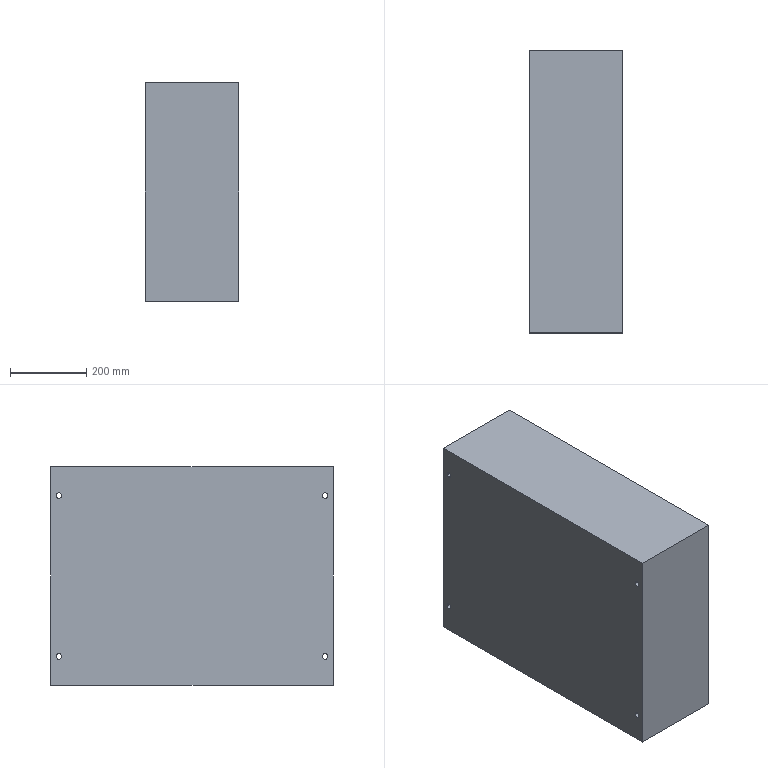Part | SolidWorks | 1 solid | 26 faces | box 246 x 742.4 x 575.6 mm | volume 104975346 mm3 | plane 14 | cylinder 12 | commonest cylinder face diameters 12 x12
STEP:
#1=CARTESIAN_POINT('',(-123.,-350.,204.));
#2=VERTEX_POINT('',#1);
#3=CARTESIAN_POINT('',(-123.,-344.,210.));
#4=VERTEX_POINT('',#3);
#5=CARTESIAN_POINT('',(-123.,-350.,210.));
#6=DIRECTION('',(1.,0.,0.));
#7=DIRECTION('',(0.,0.,-1.));
#8=AXIS2_PLACEMENT_3D('',#5,#6,#7);
#9=CIRCLE('',#8,6.);
#10=EDGE_CURVE('',#2,#4,#9,.T.);
#11=ORIENTED_EDGE('',*,*,#10,.F.);
#12=CARTESIAN_POINT('',(123.,-350.,204.));
#13=VERTEX_POINT('',#12);
#14=CARTESIAN_POINT('',(-123.,-350.,204.));
#15=DIRECTION('',(1.,0.,0.));
#16=VECTOR('',#15,1000.);
#17=LINE('',#14,#16);
#18=EDGE_CURVE('',#2,#13,#17,.T.);
#19=ORIENTED_EDGE('',*,*,#18,.T.);
#20=CARTESIAN_POINT('',(123.,-344.,210.));
#21=VERTEX_POINT('',#20);
#22=CARTESIAN_POINT('',(123.,-350.,210.));
#23=DIRECTION('',(1.,0.,0.));
#24=DIRECTION('',(0.,0.,-1.));
#25=AXIS2_PLACEMENT_3D('',#22,#23,#24);
#26=CIRCLE('',#25,6.);
#27=EDGE_CURVE('',#13,#21,#26,.T.);
#28=ORIENTED_EDGE('',*,*,#27,.T.);
#29=CARTESIAN_POINT('',(-123.,-344.,210.));
#30=DIRECTION('',(1.,0.,0.));
#31=VECTOR('',#30,1000.);
#32=LINE('',#29,#31);
#33=EDGE_CURVE('',#4,#21,#32,.T.);
#34=ORIENTED_EDGE('',*,*,#33,.F.);
#35=EDGE_LOOP('',(#11,#19,#28,#34));
#36=FACE_OUTER_BOUND('',#35,.T.);
#37=CARTESIAN_POINT('',(-123.,-350.,210.));
#38=DIRECTION('',(1.,0.,0.));
#39=DIRECTION('',(0.,0.,-1.));
#40=AXIS2_PLACEMENT_3D('',#37,#38,#39);
#41=CYLINDRICAL_SURFACE('',#40,6.);
#42=ADVANCED_FACE('',(#36),#41,.F.);
#43=CARTESIAN_POINT('',(-123.,-350.,-219.));
#44=VERTEX_POINT('',#43);
#45=CARTESIAN_POINT('',(-123.,-344.,-213.));
#46=VERTEX_POINT('',#45);
#47=CARTESIAN_POINT('',(-123.,-350.,-213.));
#48=DIRECTION('',(1.,0.,0.));
#49=DIRECTION('',(0.,0.,-1.));
#50=AXIS2_PLACEMENT_3D('',#47,#48,#49);
#51=CIRCLE('',#50,6.);
#52=EDGE_CURVE('',#44,#46,#51,.T.);
#53=ORIENTED_EDGE('',*,*,#52,.F.);
#54=CARTESIAN_POINT('',(123.,-350.,-219.));
#55=VERTEX_POINT('',#54);
#56=CARTESIAN_POINT('',(-123.,-350.,-219.));
#57=DIRECTION('',(1.,0.,0.));
#58=VECTOR('',#57,1000.);
#59=LINE('',#56,#58);
#60=EDGE_CURVE('',#44,#55,#59,.T.);
#61=ORIENTED_EDGE('',*,*,#60,.T.);
#62=CARTESIAN_POINT('',(123.,-344.,-213.));
#63=VERTEX_POINT('',#62);
#64=CARTESIAN_POINT('',(123.,-350.,-213.));
#65=DIRECTION('',(1.,0.,0.));
#66=DIRECTION('',(0.,0.,-1.));
#67=AXIS2_PLACEMENT_3D('',#64,#65,#66);
#68=CIRCLE('',#67,6.);
#69=EDGE_CURVE('',#55,#63,#68,.T.);
#70=ORIENTED_EDGE('',*,*,#69,.T.);
#71=CARTESIAN_POINT('',(-123.,-344.,-213.));
#72=DIRECTION('',(1.,0.,0.));
#73=VECTOR('',#72,1000.);
#74=LINE('',#71,#73);
#75=EDGE_CURVE('',#46,#63,#74,.T.);
#76=ORIENTED_EDGE('',*,*,#75,.F.);
#77=EDGE_LOOP('',(#53,#61,#70,#76));
#78=FACE_OUTER_BOUND('',#77,.T.);
#79=CARTESIAN_POINT('',(-123.,-350.,-213.));
#80=DIRECTION('',(1.,0.,0.));
#81=DIRECTION('',(0.,0.,-1.));
#82=AXIS2_PLACEMENT_3D('',#79,#80,#81);
#83=CYLINDRICAL_SURFACE('',#82,6.);
#84=ADVANCED_FACE('',(#78),#83,.F.);
#85=CARTESIAN_POINT('',(-123.,350.,-219.));
#86=VERTEX_POINT('',#85);
#87=CARTESIAN_POINT('',(-123.,356.,-213.));
#88=VERTEX_POINT('',#87);
#89=CARTESIAN_POINT('',(-123.,350.,-213.));
#90=DIRECTION('',(1.,0.,0.));
#91=DIRECTION('',(0.,0.,-1.));
#92=AXIS2_PLACEMENT_3D('',#89,#90,#91);
#93=CIRCLE('',#92,6.);
#94=EDGE_CURVE('',#86,#88,#93,.T.);
#95=ORIENTED_EDGE('',*,*,#94,.F.);
#96=CARTESIAN_POINT('',(123.,350.,-219.));
#97=VERTEX_POINT('',#96);
#98=CARTESIAN_POINT('',(-123.,350.,-219.));
#99=DIRECTION('',(1.,0.,0.));
#100=VECTOR('',#99,1000.);
#101=LINE('',#98,#100);
#102=EDGE_CURVE('',#86,#97,#101,.T.);
#103=ORIENTED_EDGE('',*,*,#102,.T.);
#104=CARTESIAN_POINT('',(123.,356.,-213.));
#105=VERTEX_POINT('',#104);
#106=CARTESIAN_POINT('',(123.,350.,-213.));
#107=DIRECTION('',(1.,0.,0.));
#108=DIRECTION('',(0.,0.,-1.));
#109=AXIS2_PLACEMENT_3D('',#106,#107,#108);
#110=CIRCLE('',#109,6.);
#111=EDGE_CURVE('',#97,#105,#110,.T.);
#112=ORIENTED_EDGE('',*,*,#111,.T.);
#113=CARTESIAN_POINT('',(-123.,356.,-213.));
#114=DIRECTION('',(1.,0.,0.));
#115=VECTOR('',#114,1000.);
#116=LINE('',#113,#115);
#117=EDGE_CURVE('',#88,#105,#116,.T.);
#118=ORIENTED_EDGE('',*,*,#117,.F.);
#119=EDGE_LOOP('',(#95,#103,#112,#118));
#120=FACE_OUTER_BOUND('',#119,.T.);
#121=CARTESIAN_POINT('',(-123.,350.,-213.));
#122=DIRECTION('',(1.,0.,0.));
#123=DIRECTION('',(0.,0.,-1.));
#124=AXIS2_PLACEMENT_3D('',#121,#122,#123);
#125=CYLINDRICAL_SURFACE('',#124,6.);
#126=ADVANCED_FACE('',(#120),#125,.F.);
#127=CARTESIAN_POINT('',(-123.,350.,204.));
#128=VERTEX_POINT('',#127);
#129=CARTESIAN_POINT('',(-123.,356.,210.));
#130=VERTEX_POINT('',#129);
#131=CARTESIAN_POINT('',(-123.,350.,210.));
#132=DIRECTION('',(1.,0.,0.));
#133=DIRECTION('',(0.,0.,-1.));
#134=AXIS2_PLACEMENT_3D('',#131,#132,#133);
#135=CIRCLE('',#134,6.);
#136=EDGE_CURVE('',#128,#130,#135,.T.);
#137=ORIENTED_EDGE('',*,*,#136,.F.);
#138=CARTESIAN_POINT('',(123.,350.,204.));
#139=VERTEX_POINT('',#138);
#140=CARTESIAN_POINT('',(-123.,350.,204.));
#141=DIRECTION('',(1.,0.,0.));
#142=VECTOR('',#141,1000.);
#143=LINE('',#140,#142);
#144=EDGE_CURVE('',#128,#139,#143,.T.);
#145=ORIENTED_EDGE('',*,*,#144,.T.);
#146=CARTESIAN_POINT('',(123.,356.,210.));
#147=VERTEX_POINT('',#146);
#148=CARTESIAN_POINT('',(123.,350.,210.));
#149=DIRECTION('',(1.,0.,0.));
#150=DIRECTION('',(0.,0.,-1.));
#151=AXIS2_PLACEMENT_3D('',#148,#149,#150);
#152=CIRCLE('',#151,6.);
#153=EDGE_CURVE('',#139,#147,#152,.T.);
#154=ORIENTED_EDGE('',*,*,#153,.T.);
#155=CARTESIAN_POINT('',(-123.,356.,210.));
#156=DIRECTION('',(1.,0.,0.));
#157=VECTOR('',#156,1000.);
#158=LINE('',#155,#157);
#159=EDGE_CURVE('',#130,#147,#158,.T.);
#160=ORIENTED_EDGE('',*,*,#159,.F.);
#161=EDGE_LOOP('',(#137,#145,#154,#160));
#162=FACE_OUTER_BOUND('',#161,.T.);
#163=CARTESIAN_POINT('',(-123.,350.,210.));
#164=DIRECTION('',(1.,0.,0.));
#165=DIRECTION('',(0.,0.,-1.));
#166=AXIS2_PLACEMENT_3D('',#163,#164,#165);
#167=CYLINDRICAL_SURFACE('',#166,6.);
#168=ADVANCED_FACE('',(#162),#167,.F.);
#169=CARTESIAN_POINT('',(-123.,371.2,287.8));
#170=VERTEX_POINT('',#169);
#171=CARTESIAN_POINT('',(-123.,-371.2,287.8));
#172=VERTEX_POINT('',#171);
#173=CARTESIAN_POINT('',(-123.,-371.2,287.8));
#174=DIRECTION('',(0.,-1.,0.));
#175=VECTOR('',#174,1000.);
#176=LINE('',#173,#175);
#177=EDGE_CURVE('',#170,#172,#176,.T.);
#178=ORIENTED_EDGE('',*,*,#177,.T.);
#179=CARTESIAN_POINT('',(123.,-371.2,287.8));
#180=VERTEX_POINT('',#179);
#181=CARTESIAN_POINT('',(123.,-371.2,287.8));
#182=DIRECTION('',(-1.,0.,0.));
#183=VECTOR('',#182,1000.);
#184=LINE('',#181,#183);
#185=EDGE_CURVE('',#180,#172,#184,.T.);
#186=ORIENTED_EDGE('',*,*,#185,.F.);
#187=CARTESIAN_POINT('',(123.,371.2,287.8));
#188=VERTEX_POINT('',#187);
#189=CARTESIAN_POINT('',(123.,-371.2,287.8));
#190=DIRECTION('',(0.,-1.,0.));
#191=VECTOR('',#190,1000.);
#192=LINE('',#189,#191);
#193=EDGE_CURVE('',#188,#180,#192,.T.);
#194=ORIENTED_EDGE('',*,*,#193,.F.);
#195=CARTESIAN_POINT('',(123.,371.2,287.8));
#196=DIRECTION('',(-1.,0.,0.));
#197=VECTOR('',#196,1000.);
#198=LINE('',#195,#197);
#199=EDGE_CURVE('',#188,#170,#198,.T.);
#200=ORIENTED_EDGE('',*,*,#199,.T.);
#201=EDGE_LOOP('',(#178,#186,#194,#200));
#202=FACE_OUTER_BOUND('',#201,.T.);
#203=CARTESIAN_POINT('',(123.,-371.2,287.8));
#204=DIRECTION('',(0.,0.,-1.));
#205=DIRECTION('',(-1.,0.,0.));
#206=AXIS2_PLACEMENT_3D('',#203,#204,#205);
#207=PLANE('',#206);
#208=ADVANCED_FACE('',(#202),#207,.F.);
#209=CARTESIAN_POINT('',(-123.,-371.2,-287.8));
#210=VERTEX_POINT('',#209);
#211=CARTESIAN_POINT('',(-123.,-371.2,-287.8));
#212=DIRECTION('',(0.,0.,-1.));
#213=VECTOR('',#212,1000.);
#214=LINE('',#211,#213);
#215=EDGE_CURVE('',#172,#210,#214,.T.);
#216=ORIENTED_EDGE('',*,*,#215,.T.);
#217=CARTESIAN_POINT('',(123.,-371.2,-287.8));
#218=VERTEX_POINT('',#217);
#219=CARTESIAN_POINT('',(123.,-371.2,-287.8));
#220=DIRECTION('',(-1.,0.,0.));
#221=VECTOR('',#220,1000.);
#222=LINE('',#219,#221);
#223=EDGE_CURVE('',#218,#210,#222,.T.);
#224=ORIENTED_EDGE('',*,*,#223,.F.);
#225=CARTESIAN_POINT('',(123.,-371.2,-287.8));
#226=DIRECTION('',(0.,0.,-1.));
#227=VECTOR('',#226,1000.);
#228=LINE('',#225,#227);
#229=EDGE_CURVE('',#180,#218,#228,.T.);
#230=ORIENTED_EDGE('',*,*,#229,.F.);
#231=ORIENTED_EDGE('',*,*,#185,.T.);
#232=EDGE_LOOP('',(#216,#224,#230,#231));
#233=FACE_OUTER_BOUND('',#232,.T.);
#234=CARTESIAN_POINT('',(123.,-371.2,-287.8));
#235=DIRECTION('',(0.,1.,0.));
#236=DIRECTION('',(0.,0.,1.));
#237=AXIS2_PLACEMENT_3D('',#234,#235,#236);
#238=PLANE('',#237);
#239=ADVANCED_FACE('',(#233),#238,.F.);
#240=CARTESIAN_POINT('',(-123.,371.2,-287.8));
#241=VERTEX_POINT('',#240);
#242=CARTESIAN_POINT('',(-123.,-371.2,-287.8));
#243=DIRECTION('',(0.,1.,0.));
#244=VECTOR('',#243,1000.);
#245=LINE('',#242,#244);
#246=EDGE_CURVE('',#210,#241,#245,.T.);
#247=ORIENTED_EDGE('',*,*,#246,.T.);
#248=CARTESIAN_POINT('',(123.,371.2,-287.8));
#249=VERTEX_POINT('',#248);
#250=CARTESIAN_POINT('',(123.,371.2,-287.8));
#251=DIRECTION('',(-1.,0.,0.));
#252=VECTOR('',#251,1000.);
#253=LINE('',#250,#252);
#254=EDGE_CURVE('',#249,#241,#253,.T.);
#255=ORIENTED_EDGE('',*,*,#254,.F.);
#256=CARTESIAN_POINT('',(123.,-371.2,-287.8));
#257=DIRECTION('',(0.,1.,0.));
#258=VECTOR('',#257,1000.);
#259=LINE('',#256,#258);
#260=EDGE_CURVE('',#218,#249,#259,.T.);
#261=ORIENTED_EDGE('',*,*,#260,.F.);
#262=ORIENTED_EDGE('',*,*,#223,.T.);
#263=EDGE_LOOP('',(#247,#255,#261,#262));
#264=FACE_OUTER_BOUND('',#263,.T.);
#265=CARTESIAN_POINT('',(123.,-371.2,-287.8));
#266=DIRECTION('',(0.,0.,1.));
#267=DIRECTION('',(1.,0.,0.));
#268=AXIS2_PLACEMENT_3D('',#265,#266,#267);
#269=PLANE('',#268);
#270=ADVANCED_FACE('',(#264),#269,.F.);
#271=CARTESIAN_POINT('',(-123.,371.2,-287.8));
#272=DIRECTION('',(0.,0.,1.));
#273=VECTOR('',#272,1000.);
#274=LINE('',#271,#273);
#275=EDGE_CURVE('',#241,#170,#274,.T.);
#276=ORIENTED_EDGE('',*,*,#275,.T.);
#277=ORIENTED_EDGE('',*,*,#199,.F.);
#278=CARTESIAN_POINT('',(123.,371.2,-287.8));
#279=DIRECTION('',(0.,0.,1.));
#280=VECTOR('',#279,1000.);
#281=LINE('',#278,#280);
#282=EDGE_CURVE('',#249,#188,#281,.T.);
#283=ORIENTED_EDGE('',*,*,#282,.F.);
#284=ORIENTED_EDGE('',*,*,#254,.T.);
#285=EDGE_LOOP('',(#276,#277,#283,#284));
#286=FACE_OUTER_BOUND('',#285,.T.);
#287=CARTESIAN_POINT('',(123.,371.2,-287.8));
#288=DIRECTION('',(0.,-1.,0.));
#289=DIRECTION('',(0.,0.,-1.));
#290=AXIS2_PLACEMENT_3D('',#287,#288,#289);
#291=PLANE('',#290);
#292=ADVANCED_FACE('',(#286),#291,.F.);
#293=CARTESIAN_POINT('',(123.,-344.,213.));
#294=VERTEX_POINT('',#293);
#295=CARTESIAN_POINT('',(123.,-356.,213.));
#296=VERTEX_POINT('',#295);
#297=CARTESIAN_POINT('',(123.,-350.,213.));
#298=DIRECTION('',(1.,0.,0.));
#299=DIRECTION('',(0.,0.,-1.));
#300=AXIS2_PLACEMENT_3D('',#297,#298,#299);
#301=CIRCLE('',#300,6.);
#302=EDGE_CURVE('',#294,#296,#301,.T.);
#303=ORIENTED_EDGE('',*,*,#302,.F.);
#304=CARTESIAN_POINT('',(123.,-344.,213.));
#305=DIRECTION('',(0.,0.,1.));
#306=VECTOR('',#305,1000.);
#307=LINE('',#304,#306);
#308=EDGE_CURVE('',#21,#294,#307,.T.);
#309=ORIENTED_EDGE('',*,*,#308,.F.);
#310=ORIENTED_EDGE('',*,*,#27,.F.);
#311=CARTESIAN_POINT('',(123.,-356.,210.));
#312=VERTEX_POINT('',#311);
#313=CARTESIAN_POINT('',(123.,-350.,210.));
#314=DIRECTION('',(1.,0.,0.));
#315=DIRECTION('',(0.,0.,-1.));
#316=AXIS2_PLACEMENT_3D('',#313,#314,#315);
#317=CIRCLE('',#316,6.);
#318=EDGE_CURVE('',#312,#13,#317,.T.);
#319=ORIENTED_EDGE('',*,*,#318,.F.);
#320=CARTESIAN_POINT('',(123.,-356.,213.));
#321=DIRECTION('',(0.,0.,-1.));
#322=VECTOR('',#321,1000.);
#323=LINE('',#320,#322);
#324=EDGE_CURVE('',#296,#312,#323,.T.);
#325=ORIENTED_EDGE('',*,*,#324,.F.);
#326=EDGE_LOOP('',(#303,#309,#310,#319,#325));
#327=FACE_BOUND('',#326,.T.);
#328=CARTESIAN_POINT('',(123.,-344.,-210.));
#329=VERTEX_POINT('',#328);
#330=CARTESIAN_POINT('',(123.,-356.,-210.));
#331=VERTEX_POINT('',#330);
#332=CARTESIAN_POINT('',(123.,-350.,-210.));
#333=DIRECTION('',(1.,0.,0.));
#334=DIRECTION('',(0.,0.,-1.));
#335=AXIS2_PLACEMENT_3D('',#332,#333,#334);
#336=CIRCLE('',#335,6.);
#337=EDGE_CURVE('',#329,#331,#336,.T.);
#338=ORIENTED_EDGE('',*,*,#337,.F.);
#339=CARTESIAN_POINT('',(123.,-344.,-210.));
#340=DIRECTION('',(0.,0.,1.));
#341=VECTOR('',#340,1000.);
#342=LINE('',#339,#341);
#343=EDGE_CURVE('',#63,#329,#342,.T.);
#344=ORIENTED_EDGE('',*,*,#343,.F.);
#345=ORIENTED_EDGE('',*,*,#69,.F.);
#346=CARTESIAN_POINT('',(123.,-356.,-213.));
#347=VERTEX_POINT('',#346);
#348=CARTESIAN_POINT('',(123.,-350.,-213.));
#349=DIRECTION('',(1.,0.,0.));
#350=DIRECTION('',(0.,0.,-1.));
#351=AXIS2_PLACEMENT_3D('',#348,#349,#350);
#352=CIRCLE('',#351,6.);
#353=EDGE_CURVE('',#347,#55,#352,.T.);
#354=ORIENTED_EDGE('',*,*,#353,.F.);
#355=CARTESIAN_POINT('',(123.,-356.,-210.));
#356=DIRECTION('',(0.,0.,-1.));
#357=VECTOR('',#356,1000.);
#358=LINE('',#355,#357);
#359=EDGE_CURVE('',#331,#347,#358,.T.);
#360=ORIENTED_EDGE('',*,*,#359,.F.);
#361=EDGE_LOOP('',(#338,#344,#345,#354,#360));
#362=FACE_BOUND('',#361,.T.);
#363=CARTESIAN_POINT('',(123.,356.,-210.));
#364=VERTEX_POINT('',#363);
#365=CARTESIAN_POINT('',(123.,344.,-210.));
#366=VERTEX_POINT('',#365);
#367=CARTESIAN_POINT('',(123.,350.,-210.));
#368=DIRECTION('',(1.,0.,0.));
#369=DIRECTION('',(0.,0.,-1.));
#370=AXIS2_PLACEMENT_3D('',#367,#368,#369);
#371=CIRCLE('',#370,6.);
#372=EDGE_CURVE('',#364,#366,#371,.T.);
#373=ORIENTED_EDGE('',*,*,#372,.F.);
#374=CARTESIAN_POINT('',(123.,356.,-210.));
#375=DIRECTION('',(0.,0.,1.));
#376=VECTOR('',#375,1000.);
#377=LINE('',#374,#376);
#378=EDGE_CURVE('',#105,#364,#377,.T.);
#379=ORIENTED_EDGE('',*,*,#378,.F.);
#380=ORIENTED_EDGE('',*,*,#111,.F.);
#381=CARTESIAN_POINT('',(123.,344.,-213.));
#382=VERTEX_POINT('',#381);
#383=CARTESIAN_POINT('',(123.,350.,-213.));
#384=DIRECTION('',(1.,0.,0.));
#385=DIRECTION('',(0.,0.,-1.));
#386=AXIS2_PLACEMENT_3D('',#383,#384,#385);
#387=CIRCLE('',#386,6.);
#388=EDGE_CURVE('',#382,#97,#387,.T.);
#389=ORIENTED_EDGE('',*,*,#388,.F.);
#390=CARTESIAN_POINT('',(123.,344.,-210.));
#391=DIRECTION('',(0.,0.,-1.));
#392=VECTOR('',#391,1000.);
#393=LINE('',#390,#392);
#394=EDGE_CURVE('',#366,#382,#393,.T.);
#395=ORIENTED_EDGE('',*,*,#394,.F.);
#396=EDGE_LOOP('',(#373,#379,#380,#389,#395));
#397=FACE_BOUND('',#396,.T.);
#398=CARTESIAN_POINT('',(123.,356.,213.));
#399=VERTEX_POINT('',#398);
#400=CARTESIAN_POINT('',(123.,344.,213.));
#401=VERTEX_POINT('',#400);
#402=CARTESIAN_POINT('',(123.,350.,213.));
#403=DIRECTION('',(1.,0.,0.));
#404=DIRECTION('',(0.,0.,-1.));
#405=AXIS2_PLACEMENT_3D('',#402,#403,#404);
#406=CIRCLE('',#405,6.);
#407=EDGE_CURVE('',#399,#401,#406,.T.);
#408=ORIENTED_EDGE('',*,*,#407,.F.);
#409=CARTESIAN_POINT('',(123.,356.,213.));
#410=DIRECTION('',(0.,0.,1.));
#411=VECTOR('',#410,1000.);
#412=LINE('',#409,#411);
#413=EDGE_CURVE('',#147,#399,#412,.T.);
#414=ORIENTED_EDGE('',*,*,#413,.F.);
#415=ORIENTED_EDGE('',*,*,#153,.F.);
#416=CARTESIAN_POINT('',(123.,344.,210.));
#417=VERTEX_POINT('',#416);
#418=CARTESIAN_POINT('',(123.,350.,210.));
#419=DIRECTION('',(1.,0.,0.));
#420=DIRECTION('',(0.,0.,-1.));
#421=AXIS2_PLACEMENT_3D('',#418,#419,#420);
#422=CIRCLE('',#421,6.);
#423=EDGE_CURVE('',#417,#139,#422,.T.);
#424=ORIENTED_EDGE('',*,*,#423,.F.);
#425=CARTESIAN_POINT('',(123.,344.,213.));
#426=DIRECTION('',(0.,0.,-1.));
#427=VECTOR('',#426,1000.);
#428=LINE('',#425,#427);
#429=EDGE_CURVE('',#401,#417,#428,.T.);
#430=ORIENTED_EDGE('',*,*,#429,.F.);
#431=EDGE_LOOP('',(#408,#414,#415,#424,#430));
#432=FACE_BOUND('',#431,.T.);
#433=ORIENTED_EDGE('',*,*,#193,.T.);
#434=ORIENTED_EDGE('',*,*,#229,.T.);
#435=ORIENTED_EDGE('',*,*,#260,.T.);
#436=ORIENTED_EDGE('',*,*,#282,.T.);
#437=EDGE_LOOP('',(#433,#434,#435,#436));
#438=FACE_OUTER_BOUND('',#437,.T.);
#439=CARTESIAN_POINT('',(123.,0.,0.));
#440=DIRECTION('',(1.,0.,0.));
#441=DIRECTION('',(0.,0.,-1.));
#442=AXIS2_PLACEMENT_3D('',#439,#440,#441);
#443=PLANE('',#442);
#444=ADVANCED_FACE('',(#327,#362,#397,#432,#438),#443,.T.);
#445=CARTESIAN_POINT('',(-123.,-344.,213.));
#446=VERTEX_POINT('',#445);
#447=CARTESIAN_POINT('',(-123.,-344.,213.));
#448=DIRECTION('',(0.,0.,1.));
#449=VECTOR('',#448,1000.);
#450=LINE('',#447,#449);
#451=EDGE_CURVE('',#4,#446,#450,.T.);
#452=ORIENTED_EDGE('',*,*,#451,.T.);
#453=CARTESIAN_POINT('',(-123.,-356.,213.));
#454=VERTEX_POINT('',#453);
#455=CARTESIAN_POINT('',(-123.,-350.,213.));
#456=DIRECTION('',(1.,0.,0.));
#457=DIRECTION('',(0.,0.,-1.));
#458=AXIS2_PLACEMENT_3D('',#455,#456,#457);
#459=CIRCLE('',#458,6.);
#460=EDGE_CURVE('',#446,#454,#459,.T.);
#461=ORIENTED_EDGE('',*,*,#460,.T.);
#462=CARTESIAN_POINT('',(-123.,-356.,210.));
#463=VERTEX_POINT('',#462);
#464=CARTESIAN_POINT('',(-123.,-356.,213.));
#465=DIRECTION('',(0.,0.,-1.));
#466=VECTOR('',#465,1000.);
#467=LINE('',#464,#466);
#468=EDGE_CURVE('',#454,#463,#467,.T.);
#469=ORIENTED_EDGE('',*,*,#468,.T.);
#470=CARTESIAN_POINT('',(-123.,-350.,210.));
#471=DIRECTION('',(1.,0.,0.));
#472=DIRECTION('',(0.,0.,-1.));
#473=AXIS2_PLACEMENT_3D('',#470,#471,#472);
#474=CIRCLE('',#473,6.);
#475=EDGE_CURVE('',#463,#2,#474,.T.);
#476=ORIENTED_EDGE('',*,*,#475,.T.);
#477=ORIENTED_EDGE('',*,*,#10,.T.);
#478=EDGE_LOOP('',(#452,#461,#469,#476,#477));
#479=FACE_BOUND('',#478,.T.);
#480=CARTESIAN_POINT('',(-123.,-344.,-210.));
#481=VERTEX_POINT('',#480);
#482=CARTESIAN_POINT('',(-123.,-344.,-210.));
#483=DIRECTION('',(0.,0.,1.));
#484=VECTOR('',#483,1000.);
#485=LINE('',#482,#484);
#486=EDGE_CURVE('',#46,#481,#485,.T.);
#487=ORIENTED_EDGE('',*,*,#486,.T.);
#488=CARTESIAN_POINT('',(-123.,-356.,-210.));
#489=VERTEX_POINT('',#488);
#490=CARTESIAN_POINT('',(-123.,-350.,-210.));
#491=DIRECTION('',(1.,0.,0.));
#492=DIRECTION('',(0.,0.,-1.));
#493=AXIS2_PLACEMENT_3D('',#490,#491,#492);
#494=CIRCLE('',#493,6.);
#495=EDGE_CURVE('',#481,#489,#494,.T.);
#496=ORIENTED_EDGE('',*,*,#495,.T.);
#497=CARTESIAN_POINT('',(-123.,-356.,-213.));
#498=VERTEX_POINT('',#497);
#499=CARTESIAN_POINT('',(-123.,-356.,-210.));
#500=DIRECTION('',(0.,0.,-1.));
#501=VECTOR('',#500,1000.);
#502=LINE('',#499,#501);
#503=EDGE_CURVE('',#489,#498,#502,.T.);
#504=ORIENTED_EDGE('',*,*,#503,.T.);
#505=CARTESIAN_POINT('',(-123.,-350.,-213.));
#506=DIRECTION('',(1.,0.,0.));
#507=DIRECTION('',(0.,0.,-1.));
#508=AXIS2_PLACEMENT_3D('',#505,#506,#507);
#509=CIRCLE('',#508,6.);
#510=EDGE_CURVE('',#498,#44,#509,.T.);
#511=ORIENTED_EDGE('',*,*,#510,.T.);
#512=ORIENTED_EDGE('',*,*,#52,.T.);
#513=EDGE_LOOP('',(#487,#496,#504,#511,#512));
#514=FACE_BOUND('',#513,.T.);
#515=CARTESIAN_POINT('',(-123.,356.,-210.));
#516=VERTEX_POINT('',#515);
#517=CARTESIAN_POINT('',(-123.,356.,-210.));
#518=DIRECTION('',(0.,0.,1.));
#519=VECTOR('',#518,1000.);
#520=LINE('',#517,#519);
#521=EDGE_CURVE('',#88,#516,#520,.T.);
#522=ORIENTED_EDGE('',*,*,#521,.T.);
#523=CARTESIAN_POINT('',(-123.,344.,-210.));
#524=VERTEX_POINT('',#523);
#525=CARTESIAN_POINT('',(-123.,350.,-210.));
#526=DIRECTION('',(1.,0.,0.));
#527=DIRECTION('',(0.,0.,-1.));
#528=AXIS2_PLACEMENT_3D('',#525,#526,#527);
#529=CIRCLE('',#528,6.);
#530=EDGE_CURVE('',#516,#524,#529,.T.);
#531=ORIENTED_EDGE('',*,*,#530,.T.);
#532=CARTESIAN_POINT('',(-123.,344.,-213.));
#533=VERTEX_POINT('',#532);
#534=CARTESIAN_POINT('',(-123.,344.,-210.));
#535=DIRECTION('',(0.,0.,-1.));
#536=VECTOR('',#535,1000.);
#537=LINE('',#534,#536);
#538=EDGE_CURVE('',#524,#533,#537,.T.);
#539=ORIENTED_EDGE('',*,*,#538,.T.);
#540=CARTESIAN_POINT('',(-123.,350.,-213.));
#541=DIRECTION('',(1.,0.,0.));
#542=DIRECTION('',(0.,0.,-1.));
#543=AXIS2_PLACEMENT_3D('',#540,#541,#542);
#544=CIRCLE('',#543,6.);
#545=EDGE_CURVE('',#533,#86,#544,.T.);
#546=ORIENTED_EDGE('',*,*,#545,.T.);
#547=ORIENTED_EDGE('',*,*,#94,.T.);
#548=EDGE_LOOP('',(#522,#531,#539,#546,#547));
#549=FACE_BOUND('',#548,.T.);
#550=CARTESIAN_POINT('',(-123.,356.,213.));
#551=VERTEX_POINT('',#550);
#552=CARTESIAN_POINT('',(-123.,356.,213.));
#553=DIRECTION('',(0.,0.,1.));
#554=VECTOR('',#553,1000.);
#555=LINE('',#552,#554);
#556=EDGE_CURVE('',#130,#551,#555,.T.);
#557=ORIENTED_EDGE('',*,*,#556,.T.);
#558=CARTESIAN_POINT('',(-123.,344.,213.));
#559=VERTEX_POINT('',#558);
#560=CARTESIAN_POINT('',(-123.,350.,213.));
#561=DIRECTION('',(1.,0.,0.));
#562=DIRECTION('',(0.,0.,-1.));
#563=AXIS2_PLACEMENT_3D('',#560,#561,#562);
#564=CIRCLE('',#563,6.);
#565=EDGE_CURVE('',#551,#559,#564,.T.);
#566=ORIENTED_EDGE('',*,*,#565,.T.);
#567=CARTESIAN_POINT('',(-123.,344.,210.));
#568=VERTEX_POINT('',#567);
#569=CARTESIAN_POINT('',(-123.,344.,213.));
#570=DIRECTION('',(0.,0.,-1.));
#571=VECTOR('',#570,1000.);
#572=LINE('',#569,#571);
#573=EDGE_CURVE('',#559,#568,#572,.T.);
#574=ORIENTED_EDGE('',*,*,#573,.T.);
#575=CARTESIAN_POINT('',(-123.,350.,210.));
#576=DIRECTION('',(1.,0.,0.));
#577=DIRECTION('',(0.,0.,-1.));
#578=AXIS2_PLACEMENT_3D('',#575,#576,#577);
#579=CIRCLE('',#578,6.);
#580=EDGE_CURVE('',#568,#128,#579,.T.);
#581=ORIENTED_EDGE('',*,*,#580,.T.);
#582=ORIENTED_EDGE('',*,*,#136,.T.);
#583=EDGE_LOOP('',(#557,#566,#574,#581,#582));
#584=FACE_BOUND('',#583,.T.);
#585=ORIENTED_EDGE('',*,*,#177,.F.);
#586=ORIENTED_EDGE('',*,*,#275,.F.);
#587=ORIENTED_EDGE('',*,*,#246,.F.);
#588=ORIENTED_EDGE('',*,*,#215,.F.);
#589=EDGE_LOOP('',(#585,#586,#587,#588));
#590=FACE_OUTER_BOUND('',#589,.T.);
#591=CARTESIAN_POINT('',(-123.,0.,0.));
#592=DIRECTION('',(1.,0.,0.));
#593=DIRECTION('',(0.,0.,-1.));
#594=AXIS2_PLACEMENT_3D('',#591,#592,#593);
#595=PLANE('',#594);
#596=ADVANCED_FACE('',(#479,#514,#549,#584,#590),#595,.F.);
#597=ORIENTED_EDGE('',*,*,#407,.T.);
#598=CARTESIAN_POINT('',(-123.,344.,213.));
#599=DIRECTION('',(1.,0.,0.));
#600=VECTOR('',#599,1000.);
#601=LINE('',#598,#600);
#602=EDGE_CURVE('',#559,#401,#601,.T.);
#603=ORIENTED_EDGE('',*,*,#602,.F.);
#604=ORIENTED_EDGE('',*,*,#565,.F.);
#605=CARTESIAN_POINT('',(-123.,356.,213.));
#606=DIRECTION('',(1.,0.,0.));
#607=VECTOR('',#606,1000.);
#608=LINE('',#605,#607);
#609=EDGE_CURVE('',#551,#399,#608,.T.);
#610=ORIENTED_EDGE('',*,*,#609,.T.);
#611=EDGE_LOOP('',(#597,#603,#604,#610));
#612=FACE_OUTER_BOUND('',#611,.T.);
#613=CARTESIAN_POINT('',(-123.,350.,213.));
#614=DIRECTION('',(1.,0.,0.));
#615=DIRECTION('',(0.,0.,-1.));
#616=AXIS2_PLACEMENT_3D('',#613,#614,#615);
#617=CYLINDRICAL_SURFACE('',#616,6.);
#618=ADVANCED_FACE('',(#612),#617,.F.);
#619=ORIENTED_EDGE('',*,*,#413,.T.);
#620=ORIENTED_EDGE('',*,*,#609,.F.);
#621=ORIENTED_EDGE('',*,*,#556,.F.);
#622=ORIENTED_EDGE('',*,*,#159,.T.);
#623=EDGE_LOOP('',(#619,#620,#621,#622));
#624=FACE_OUTER_BOUND('',#623,.T.);
#625=CARTESIAN_POINT('',(-123.,356.,213.));
#626=DIRECTION('',(0.,1.,0.));
#627=DIRECTION('',(0.,0.,1.));
#628=AXIS2_PLACEMENT_3D('',#625,#626,#627);
#629=PLANE('',#628);
#630=ADVANCED_FACE('',(#624),#629,.F.);
#631=ORIENTED_EDGE('',*,*,#144,.F.);
#632=ORIENTED_EDGE('',*,*,#580,.F.);
#633=CARTESIAN_POINT('',(-123.,344.,210.));
#634=DIRECTION('',(1.,0.,0.));
#635=VECTOR('',#634,1000.);
#636=LINE('',#633,#635);
#637=EDGE_CURVE('',#568,#417,#636,.T.);
#638=ORIENTED_EDGE('',*,*,#637,.T.);
#639=ORIENTED_EDGE('',*,*,#423,.T.);
#640=EDGE_LOOP('',(#631,#632,#638,#639));
#641=FACE_OUTER_BOUND('',#640,.T.);
#642=CARTESIAN_POINT('',(-123.,350.,210.));
#643=DIRECTION('',(1.,0.,0.));
#644=DIRECTION('',(0.,0.,-1.));
#645=AXIS2_PLACEMENT_3D('',#642,#643,#644);
#646=CYLINDRICAL_SURFACE('',#645,6.);
#647=ADVANCED_FACE('',(#641),#646,.F.);
#648=ORIENTED_EDGE('',*,*,#429,.T.);
#649=ORIENTED_EDGE('',*,*,#637,.F.);
#650=ORIENTED_EDGE('',*,*,#573,.F.);
#651=ORIENTED_EDGE('',*,*,#602,.T.);
#652=EDGE_LOOP('',(#648,#649,#650,#651));
#653=FACE_OUTER_BOUND('',#652,.T.);
#654=CARTESIAN_POINT('',(-123.,344.,213.));
#655=DIRECTION('',(0.,-1.,0.));
#656=DIRECTION('',(0.,0.,-1.));
#657=AXIS2_PLACEMENT_3D('',#654,#655,#656);
#658=PLANE('',#657);
#659=ADVANCED_FACE('',(#653),#658,.F.);
#660=ORIENTED_EDGE('',*,*,#372,.T.);
#661=CARTESIAN_POINT('',(-123.,344.,-210.));
#662=DIRECTION('',(1.,0.,0.));
#663=VECTOR('',#662,1000.);
#664=LINE('',#661,#663);
#665=EDGE_CURVE('',#524,#366,#664,.T.);
#666=ORIENTED_EDGE('',*,*,#665,.F.);
#667=ORIENTED_EDGE('',*,*,#530,.F.);
#668=CARTESIAN_POINT('',(-123.,356.,-210.));
#669=DIRECTION('',(1.,0.,0.));
#670=VECTOR('',#669,1000.);
#671=LINE('',#668,#670);
#672=EDGE_CURVE('',#516,#364,#671,.T.);
#673=ORIENTED_EDGE('',*,*,#672,.T.);
#674=EDGE_LOOP('',(#660,#666,#667,#673));
#675=FACE_OUTER_BOUND('',#674,.T.);
#676=CARTESIAN_POINT('',(-123.,350.,-210.));
#677=DIRECTION('',(1.,0.,0.));
#678=DIRECTION('',(0.,0.,-1.));
#679=AXIS2_PLACEMENT_3D('',#676,#677,#678);
#680=CYLINDRICAL_SURFACE('',#679,6.);
#681=ADVANCED_FACE('',(#675),#680,.F.);
#682=ORIENTED_EDGE('',*,*,#378,.T.);
#683=ORIENTED_EDGE('',*,*,#672,.F.);
#684=ORIENTED_EDGE('',*,*,#521,.F.);
#685=ORIENTED_EDGE('',*,*,#117,.T.);
#686=EDGE_LOOP('',(#682,#683,#684,#685));
#687=FACE_OUTER_BOUND('',#686,.T.);
#688=CARTESIAN_POINT('',(-123.,356.,-210.));
#689=DIRECTION('',(0.,1.,0.));
#690=DIRECTION('',(0.,0.,1.));
#691=AXIS2_PLACEMENT_3D('',#688,#689,#690);
#692=PLANE('',#691);
#693=ADVANCED_FACE('',(#687),#692,.F.);
#694=ORIENTED_EDGE('',*,*,#102,.F.);
#695=ORIENTED_EDGE('',*,*,#545,.F.);
#696=CARTESIAN_POINT('',(-123.,344.,-213.));
#697=DIRECTION('',(1.,0.,0.));
#698=VECTOR('',#697,1000.);
#699=LINE('',#696,#698);
#700=EDGE_CURVE('',#533,#382,#699,.T.);
#701=ORIENTED_EDGE('',*,*,#700,.T.);
#702=ORIENTED_EDGE('',*,*,#388,.T.);
#703=EDGE_LOOP('',(#694,#695,#701,#702));
#704=FACE_OUTER_BOUND('',#703,.T.);
#705=CARTESIAN_POINT('',(-123.,350.,-213.));
#706=DIRECTION('',(1.,0.,0.));
#707=DIRECTION('',(0.,0.,-1.));
#708=AXIS2_PLACEMENT_3D('',#705,#706,#707);
#709=CYLINDRICAL_SURFACE('',#708,6.);
#710=ADVANCED_FACE('',(#704),#709,.F.);
#711=ORIENTED_EDGE('',*,*,#394,.T.);
#712=ORIENTED_EDGE('',*,*,#700,.F.);
#713=ORIENTED_EDGE('',*,*,#538,.F.);
#714=ORIENTED_EDGE('',*,*,#665,.T.);
#715=EDGE_LOOP('',(#711,#712,#713,#714));
#716=FACE_OUTER_BOUND('',#715,.T.);
#717=CARTESIAN_POINT('',(-123.,344.,-210.));
#718=DIRECTION('',(0.,-1.,0.));
#719=DIRECTION('',(0.,0.,-1.));
#720=AXIS2_PLACEMENT_3D('',#717,#718,#719);
#721=PLANE('',#720);
#722=ADVANCED_FACE('',(#716),#721,.F.);
#723=ORIENTED_EDGE('',*,*,#337,.T.);
#724=CARTESIAN_POINT('',(-123.,-356.,-210.));
#725=DIRECTION('',(1.,0.,0.));
#726=VECTOR('',#725,1000.);
#727=LINE('',#724,#726);
#728=EDGE_CURVE('',#489,#331,#727,.T.);
#729=ORIENTED_EDGE('',*,*,#728,.F.);
#730=ORIENTED_EDGE('',*,*,#495,.F.);
#731=CARTESIAN_POINT('',(-123.,-344.,-210.));
#732=DIRECTION('',(1.,0.,0.));
#733=VECTOR('',#732,1000.);
#734=LINE('',#731,#733);
#735=EDGE_CURVE('',#481,#329,#734,.T.);
#736=ORIENTED_EDGE('',*,*,#735,.T.);
#737=EDGE_LOOP('',(#723,#729,#730,#736));
#738=FACE_OUTER_BOUND('',#737,.T.);
#739=CARTESIAN_POINT('',(-123.,-350.,-210.));
#740=DIRECTION('',(1.,0.,0.));
#741=DIRECTION('',(0.,0.,-1.));
#742=AXIS2_PLACEMENT_3D('',#739,#740,#741);
#743=CYLINDRICAL_SURFACE('',#742,6.);
#744=ADVANCED_FACE('',(#738),#743,.F.);
#745=ORIENTED_EDGE('',*,*,#343,.T.);
#746=ORIENTED_EDGE('',*,*,#735,.F.);
#747=ORIENTED_EDGE('',*,*,#486,.F.);
#748=ORIENTED_EDGE('',*,*,#75,.T.);
#749=EDGE_LOOP('',(#745,#746,#747,#748));
#750=FACE_OUTER_BOUND('',#749,.T.);
#751=CARTESIAN_POINT('',(-123.,-344.,-210.));
#752=DIRECTION('',(0.,1.,0.));
#753=DIRECTION('',(0.,0.,1.));
#754=AXIS2_PLACEMENT_3D('',#751,#752,#753);
#755=PLANE('',#754);
#756=ADVANCED_FACE('',(#750),#755,.F.);
#757=ORIENTED_EDGE('',*,*,#60,.F.);
#758=ORIENTED_EDGE('',*,*,#510,.F.);
#759=CARTESIAN_POINT('',(-123.,-356.,-213.));
#760=DIRECTION('',(1.,0.,0.));
#761=VECTOR('',#760,1000.);
#762=LINE('',#759,#761);
#763=EDGE_CURVE('',#498,#347,#762,.T.);
#764=ORIENTED_EDGE('',*,*,#763,.T.);
#765=ORIENTED_EDGE('',*,*,#353,.T.);
#766=EDGE_LOOP('',(#757,#758,#764,#765));
#767=FACE_OUTER_BOUND('',#766,.T.);
#768=CARTESIAN_POINT('',(-123.,-350.,-213.));
#769=DIRECTION('',(1.,0.,0.));
#770=DIRECTION('',(0.,0.,-1.));
#771=AXIS2_PLACEMENT_3D('',#768,#769,#770);
#772=CYLINDRICAL_SURFACE('',#771,6.);
#773=ADVANCED_FACE('',(#767),#772,.F.);
#774=ORIENTED_EDGE('',*,*,#359,.T.);
#775=ORIENTED_EDGE('',*,*,#763,.F.);
#776=ORIENTED_EDGE('',*,*,#503,.F.);
#777=ORIENTED_EDGE('',*,*,#728,.T.);
#778=EDGE_LOOP('',(#774,#775,#776,#777));
#779=FACE_OUTER_BOUND('',#778,.T.);
#780=CARTESIAN_POINT('',(-123.,-356.,-210.));
#781=DIRECTION('',(0.,-1.,0.));
#782=DIRECTION('',(0.,0.,-1.));
#783=AXIS2_PLACEMENT_3D('',#780,#781,#782);
#784=PLANE('',#783);
#785=ADVANCED_FACE('',(#779),#784,.F.);
#786=ORIENTED_EDGE('',*,*,#302,.T.);
#787=CARTESIAN_POINT('',(-123.,-356.,213.));
#788=DIRECTION('',(1.,0.,0.));
#789=VECTOR('',#788,1000.);
#790=LINE('',#787,#789);
#791=EDGE_CURVE('',#454,#296,#790,.T.);
#792=ORIENTED_EDGE('',*,*,#791,.F.);
#793=ORIENTED_EDGE('',*,*,#460,.F.);
#794=CARTESIAN_POINT('',(-123.,-344.,213.));
#795=DIRECTION('',(1.,0.,0.));
#796=VECTOR('',#795,1000.);
#797=LINE('',#794,#796);
#798=EDGE_CURVE('',#446,#294,#797,.T.);
#799=ORIENTED_EDGE('',*,*,#798,.T.);
#800=EDGE_LOOP('',(#786,#792,#793,#799));
#801=FACE_OUTER_BOUND('',#800,.T.);
#802=CARTESIAN_POINT('',(-123.,-350.,213.));
#803=DIRECTION('',(1.,0.,0.));
#804=DIRECTION('',(0.,0.,-1.));
#805=AXIS2_PLACEMENT_3D('',#802,#803,#804);
#806=CYLINDRICAL_SURFACE('',#805,6.);
#807=ADVANCED_FACE('',(#801),#806,.F.);
#808=ORIENTED_EDGE('',*,*,#308,.T.);
#809=ORIENTED_EDGE('',*,*,#798,.F.);
#810=ORIENTED_EDGE('',*,*,#451,.F.);
#811=ORIENTED_EDGE('',*,*,#33,.T.);
#812=EDGE_LOOP('',(#808,#809,#810,#811));
#813=FACE_OUTER_BOUND('',#812,.T.);
#814=CARTESIAN_POINT('',(-123.,-344.,213.));
#815=DIRECTION('',(0.,1.,0.));
#816=DIRECTION('',(0.,0.,1.));
#817=AXIS2_PLACEMENT_3D('',#814,#815,#816);
#818=PLANE('',#817);
#819=ADVANCED_FACE('',(#813),#818,.F.);
#820=ORIENTED_EDGE('',*,*,#18,.F.);
#821=ORIENTED_EDGE('',*,*,#475,.F.);
#822=CARTESIAN_POINT('',(-123.,-356.,210.));
#823=DIRECTION('',(1.,0.,0.));
#824=VECTOR('',#823,1000.);
#825=LINE('',#822,#824);
#826=EDGE_CURVE('',#463,#312,#825,.T.);
#827=ORIENTED_EDGE('',*,*,#826,.T.);
#828=ORIENTED_EDGE('',*,*,#318,.T.);
#829=EDGE_LOOP('',(#820,#821,#827,#828));
#830=FACE_OUTER_BOUND('',#829,.T.);
#831=CARTESIAN_POINT('',(-123.,-350.,210.));
#832=DIRECTION('',(1.,0.,0.));
#833=DIRECTION('',(0.,0.,-1.));
#834=AXIS2_PLACEMENT_3D('',#831,#832,#833);
#835=CYLINDRICAL_SURFACE('',#834,6.);
#836=ADVANCED_FACE('',(#830),#835,.F.);
#837=ORIENTED_EDGE('',*,*,#324,.T.);
#838=ORIENTED_EDGE('',*,*,#826,.F.);
#839=ORIENTED_EDGE('',*,*,#468,.F.);
#840=ORIENTED_EDGE('',*,*,#791,.T.);
#841=EDGE_LOOP('',(#837,#838,#839,#840));
#842=FACE_OUTER_BOUND('',#841,.T.);
#843=CARTESIAN_POINT('',(-123.,-356.,213.));
#844=DIRECTION('',(0.,-1.,0.));
#845=DIRECTION('',(0.,0.,-1.));
#846=AXIS2_PLACEMENT_3D('',#843,#844,#845);
#847=PLANE('',#846);
#848=ADVANCED_FACE('',(#842),#847,.F.);
#849=CLOSED_SHELL('',(#42,#84,#126,#168,#208,#239,#270,#292,#444,#596,#618,#630,#647,#659,#681,#693,#710,#722,#744,#756,#773,#785,#807,#819,#836,#848));
#850=MANIFOLD_SOLID_BREP('',#849);
#851=CARTESIAN_POINT('',(0.,0.,0.));
#852=DIRECTION('',(0.,0.,1.));
#853=DIRECTION('',(1.,0.,0.));
#854=AXIS2_PLACEMENT_3D('',#851,#852,#853);
#855=(LENGTH_UNIT()NAMED_UNIT(*)SI_UNIT(.MILLI.,.METRE.));
#856=UNCERTAINTY_MEASURE_WITH_UNIT(LENGTH_MEASURE(0.00001),#855,'','');
#857=(NAMED_UNIT(*)PLANE_ANGLE_UNIT()SI_UNIT($,.RADIAN.));
#858=(NAMED_UNIT(*)SI_UNIT($,.STERADIAN.)SOLID_ANGLE_UNIT());
#859=(GEOMETRIC_REPRESENTATION_CONTEXT(3)GLOBAL_UNCERTAINTY_ASSIGNED_CONTEXT((#856))GLOBAL_UNIT_ASSIGNED_CONTEXT((#855,#857,#858))REPRESENTATION_CONTEXT('',''));
#860=ADVANCED_BREP_SHAPE_REPRESENTATION('',(#850,#854),#859);